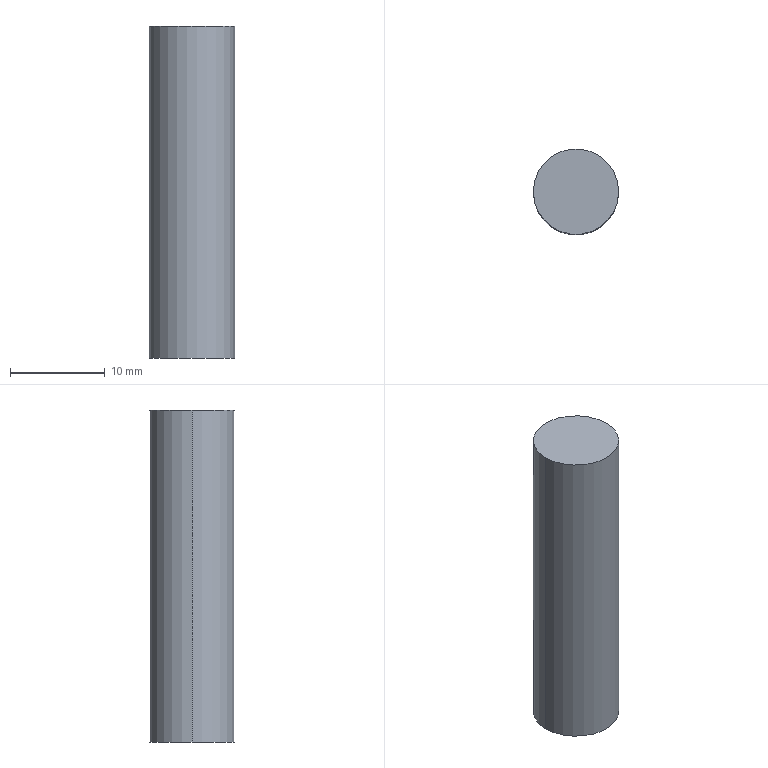Part | SolidWorks | features BaseBody 1 | 1 solid | 4 faces | box 9 x 9 x 35 mm | volume 2227 mm3 | cylinder 2 | plane 2 | commonest cylinder face diameters 9 x2
STEP:
#1=CARTESIAN_POINT('',(50.5,190.,-40.));
#2=VERTEX_POINT('',#1);
#3=CARTESIAN_POINT('',(41.5,190.,-40.));
#4=VERTEX_POINT('',#3);
#5=CARTESIAN_POINT('',(46.,190.,-40.));
#6=DIRECTION('',(0.,0.,1.));
#7=DIRECTION('',(-1.,0.,0.));
#8=AXIS2_PLACEMENT_3D('',#5,#6,#7);
#9=CIRCLE('',#8,4.5);
#10=EDGE_CURVE('',#2,#4,#9,.T.);
#11=ORIENTED_EDGE('',*,*,#10,.F.);
#12=CARTESIAN_POINT('',(50.5,190.,-75.));
#13=VERTEX_POINT('',#12);
#14=CARTESIAN_POINT('',(50.5,190.,-40.));
#15=DIRECTION('',(0.,0.,-1.));
#16=VECTOR('',#15,1000.);
#17=LINE('',#14,#16);
#18=EDGE_CURVE('',#2,#13,#17,.T.);
#19=ORIENTED_EDGE('',*,*,#18,.T.);
#20=CARTESIAN_POINT('',(41.5,190.,-75.));
#21=VERTEX_POINT('',#20);
#22=CARTESIAN_POINT('',(46.,190.,-75.));
#23=DIRECTION('',(0.,0.,1.));
#24=DIRECTION('',(-1.,0.,0.));
#25=AXIS2_PLACEMENT_3D('',#22,#23,#24);
#26=CIRCLE('',#25,4.5);
#27=EDGE_CURVE('',#13,#21,#26,.T.);
#28=ORIENTED_EDGE('',*,*,#27,.T.);
#29=CARTESIAN_POINT('',(41.5,190.,-40.));
#30=DIRECTION('',(0.,0.,-1.));
#31=VECTOR('',#30,1000.);
#32=LINE('',#29,#31);
#33=EDGE_CURVE('',#4,#21,#32,.T.);
#34=ORIENTED_EDGE('',*,*,#33,.F.);
#35=EDGE_LOOP('',(#11,#19,#28,#34));
#36=FACE_OUTER_BOUND('',#35,.T.);
#37=CARTESIAN_POINT('',(46.,190.,-40.));
#38=DIRECTION('',(0.,0.,-1.));
#39=DIRECTION('',(-1.,0.,0.));
#40=AXIS2_PLACEMENT_3D('',#37,#38,#39);
#41=CYLINDRICAL_SURFACE('',#40,4.5);
#42=ADVANCED_FACE('',(#36),#41,.T.);
#43=ORIENTED_EDGE('',*,*,#18,.F.);
#44=CARTESIAN_POINT('',(46.,190.,-40.));
#45=DIRECTION('',(0.,0.,1.));
#46=DIRECTION('',(-1.,0.,0.));
#47=AXIS2_PLACEMENT_3D('',#44,#45,#46);
#48=CIRCLE('',#47,4.5);
#49=EDGE_CURVE('',#4,#2,#48,.T.);
#50=ORIENTED_EDGE('',*,*,#49,.F.);
#51=ORIENTED_EDGE('',*,*,#33,.T.);
#52=CARTESIAN_POINT('',(46.,190.,-75.));
#53=DIRECTION('',(0.,0.,1.));
#54=DIRECTION('',(-1.,0.,0.));
#55=AXIS2_PLACEMENT_3D('',#52,#53,#54);
#56=CIRCLE('',#55,4.5);
#57=EDGE_CURVE('',#21,#13,#56,.T.);
#58=ORIENTED_EDGE('',*,*,#57,.T.);
#59=EDGE_LOOP('',(#43,#50,#51,#58));
#60=FACE_OUTER_BOUND('',#59,.T.);
#61=CARTESIAN_POINT('',(46.,190.,-40.));
#62=DIRECTION('',(0.,0.,-1.));
#63=DIRECTION('',(-1.,0.,0.));
#64=AXIS2_PLACEMENT_3D('',#61,#62,#63);
#65=CYLINDRICAL_SURFACE('',#64,4.5);
#66=ADVANCED_FACE('',(#60),#65,.T.);
#67=ORIENTED_EDGE('',*,*,#49,.T.);
#68=ORIENTED_EDGE('',*,*,#10,.T.);
#69=EDGE_LOOP('',(#67,#68));
#70=FACE_OUTER_BOUND('',#69,.T.);
#71=CARTESIAN_POINT('',(46.,190.,-40.));
#72=DIRECTION('',(0.,0.,1.));
#73=DIRECTION('',(1.,0.,0.));
#74=AXIS2_PLACEMENT_3D('',#71,#72,#73);
#75=PLANE('',#74);
#76=ADVANCED_FACE('',(#70),#75,.T.);
#77=ORIENTED_EDGE('',*,*,#57,.F.);
#78=ORIENTED_EDGE('',*,*,#27,.F.);
#79=EDGE_LOOP('',(#77,#78));
#80=FACE_OUTER_BOUND('',#79,.T.);
#81=CARTESIAN_POINT('',(46.,190.,-75.));
#82=DIRECTION('',(0.,0.,1.));
#83=DIRECTION('',(1.,0.,0.));
#84=AXIS2_PLACEMENT_3D('',#81,#82,#83);
#85=PLANE('',#84);
#86=ADVANCED_FACE('',(#80),#85,.F.);
#87=CLOSED_SHELL('',(#42,#66,#76,#86));
#88=MANIFOLD_SOLID_BREP('',#87);
#89=CARTESIAN_POINT('',(0.,0.,0.));
#90=DIRECTION('',(0.,0.,1.));
#91=DIRECTION('',(1.,0.,0.));
#92=AXIS2_PLACEMENT_3D('',#89,#90,#91);
#93=(LENGTH_UNIT()NAMED_UNIT(*)SI_UNIT(.MILLI.,.METRE.));
#94=UNCERTAINTY_MEASURE_WITH_UNIT(LENGTH_MEASURE(0.00001),#93,'','');
#95=(NAMED_UNIT(*)PLANE_ANGLE_UNIT()SI_UNIT($,.RADIAN.));
#96=(NAMED_UNIT(*)SI_UNIT($,.STERADIAN.)SOLID_ANGLE_UNIT());
#97=(GEOMETRIC_REPRESENTATION_CONTEXT(3)GLOBAL_UNCERTAINTY_ASSIGNED_CONTEXT((#94))GLOBAL_UNIT_ASSIGNED_CONTEXT((#93,#95,#96))REPRESENTATION_CONTEXT('',''));
#98=ADVANCED_BREP_SHAPE_REPRESENTATION('',(#88,#92),#97);